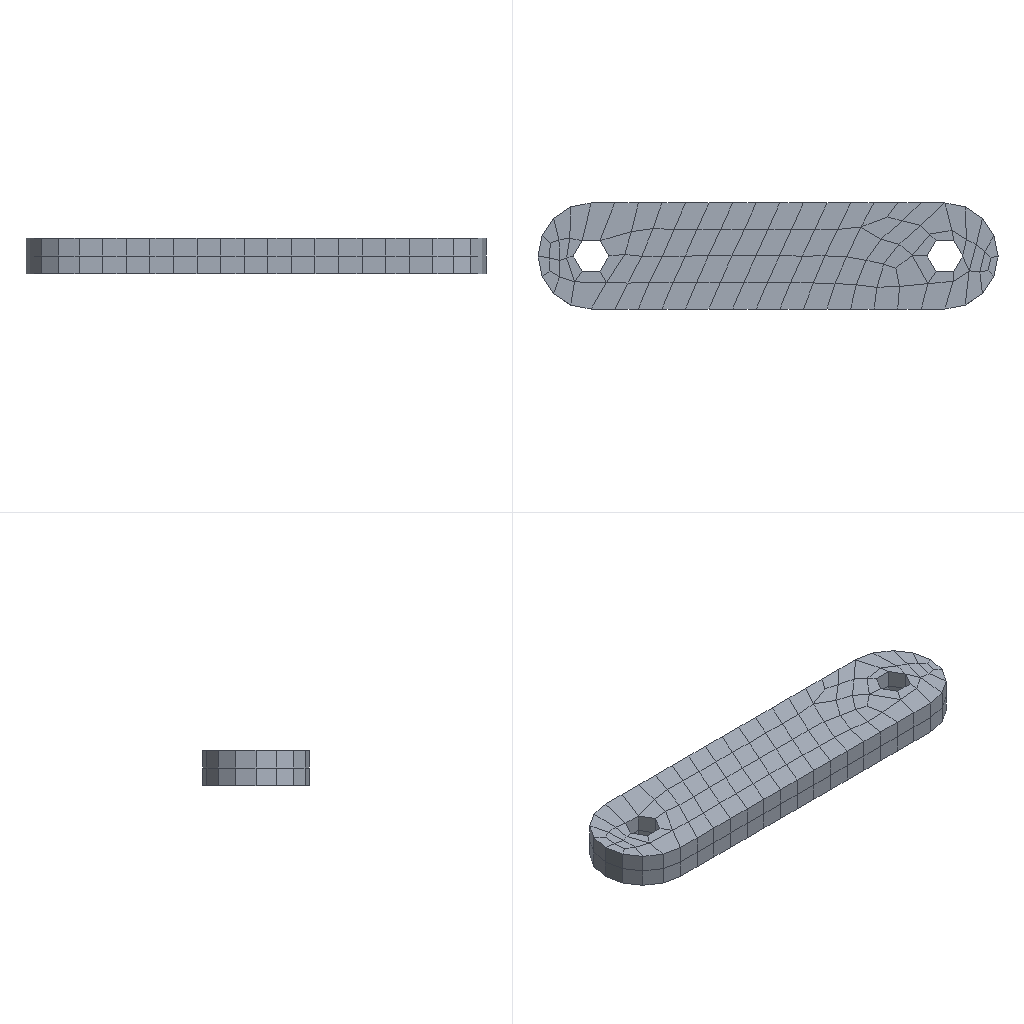Simulation study | ansys workbench
Ansys APDL input file, long lists of numbers shortened:
/batch
/config,noeldb,1     ! force off writing results to database
*get,_wallstrt,active,,time,wall
! ANSYS input file written by Workbench version 2022 R1
! File used for geometry attach: F:\ansys（分析文件汇总)\连杆和曲柄有限元分析\舵机架.STEP
/title,wbnew--____ (B5)
! ****** Begin Custom Load Command Snippet ******
/COM, ACT Extensions:
/COM,     LSDYNA, 2021.1
/COM,
! ****** End   Custom Load Command Snippet ******
*DIM,_wb_ProjectScratch_dir,string,248
_wb_ProjectScratch_dir(1) = 'C:\Users\Administrator\AppData\Local\Temp\WB_Administrator_9524_2\_ProjectScratch\ScrD814\'
*DIM,_wb_SolverFiles_dir,string,248
_wb_SolverFiles_dir(1) = 'C:\Users\Administrator\AppData\Local\Temp\WB_Administrator_9524_2\wbnew_files\dp0\SYS\MECH\'
*DIM,_wb_userfiles_dir,string,248
_wb_userfiles_dir(1) = 'C:\Users\Administrator\AppData\Local\Temp\WB_Administrator_9524_2\wbnew_files\user_files\'
/com,--- Data in consistent NMM units. See Solving Units in the help system for more information.
/units,MPA
/nopr
/wb,file,start              !  signify a WB generated input file
/prep7
! Turn off shape checking because checks already performed inside WB mesher.
! See help system for more information.
SHPP,OFF,,NOWARN
/nolist
etcon,set             ! allow ANSYS to choose best KEYOP's for 180x elements, resets any applicable keyopt to MAPDL defaults
/com,*********** Nodes for the whole assembly ***********
nblock,3,,114635
(1i9,3e20.9e3)
        1     5.800000000E+00     2.000000000E+01    -4.000000000E+00
! (104213 more lines like these left out)
-1
/wb,elem,start            !  set before creation of elements
/com,*********** Elements for Body 1 "___-FreeParts|____-____5" ***********
et,1,187
eblock,19,solid,,30033
(19i9)
        1        1        1        1        0        0        0        0       10        0    29225    57461    59689    58819    57715    94284   102448    94278    94275
! (60065 more lines like these left out)
-1
/com,*********** Elements for Body 2 "___-FreeParts|____-____1" ***********
et,2,187
eblock,19,solid,,29224
(19i9)
        2        2        2        2        0        0        0        0       10        0        1     6994     7254     8134     7776    47665    49608    47675    47673
! (58447 more lines like these left out)
-1
/wb,elem,end               !  done creating elements
/com,*********** Send User Defined Coordinate System(s) ***********
csys,0
toffst,273.15,  ! Temperature offset from absolute zero
/com,*********** Set Reference Temperature ***********
tref,22.
/wb,mat,start              !  starting to send materials
/com,*********** Send Materials ***********
Temperature = 'TEMP' ! Temperature
MP,DENS,1,1.25e-09,	! tonne mm^-3
MP,ALPX,1,1.2e-05,	! C^-1
MP,C,1,434000000,	! mm^2 s^-2 C^-1
MP,KXX,1,60.5,	! tonne mm s^-3 C^-1
MP,RSVX,1,0.00017,	! ohm mm
MP,EX,1,3000,	! tonne s^-2 mm^-1
MP,NUXY,1,0.3,
MP,MURX,1,10000,
Temperature = 'TEMP' ! Temperature
MP,DENS,2,1.25e-09,	! tonne mm^-3
MP,ALPX,2,1.2e-05,	! C^-1
MP,C,2,434000000,	! mm^2 s^-2 C^-1
MP,KXX,2,60.5,	! tonne mm s^-3 C^-1
MP,RSVX,2,0.00017,	! ohm mm
MP,EX,2,3000,	! tonne s^-2 mm^-1
MP,NUXY,2,0.3,
MP,MURX,2,10000,
/wb,mat,end                !  done sending materials
!************************* Model Summary ********************
!___-FreeParts|____-____5,	PLA,	matid,	1
!___-FreeParts|____-____1,	PLA,	matid,	2
!************************* End Model Summary ********************
! get the diagonal of the bounding box. Needed later for other things
*get,_xmin,node,,mnloc,x
*get,_ymin,node,,mnloc,y
*get,_zmin,node,,mnloc,z
*get,_xmax,node,,mxloc,x
*get,_ymax,node,,mxloc,y
*get,_zmax,node,,mxloc,z
_ASMDIAG=(_xmax-_xmin)*(_xmax-_xmin)+(_ymax-_ymin)*(_ymax-_ymin)+(_zmax-_zmin)*(_zmax-_zmin)
_ASMDIAG=SQRT(_ASMDIAG)
/wb,contact,start          !  starting to send contact
/com,*********** Create Contact "接触区域" ***********
/com,            Real Constant Set For Above Contact Is 4 & 3
*set,tid,4
*set,cid,3
r,tid
r,cid
et,tid,170
et,cid,174
eblock,10,,,2211
(15i9)
    83154        4        4        4        0    51462    51466    52017    52017    60587    60624    52017    60589
! (2210 more lines like these left out)
-1
eblock,10,,,2211
(15i9)
    85365        3        3        3        0    51462    51466    52017    52017    60587    60624    52017    60589
! (2210 more lines like these left out)
-1
eblock,10,,,2299
(15i9)
    87576        3        4        3        0     3099     3412     3676     3676    25484    27890     3676    25487
! (2298 more lines like these left out)
-1
eblock,10,,,2299
(15i9)
    89875        4        3        4        0     3099     3412     3676     3676    25484    27890     3676    25487
! (2298 more lines like these left out)
-1
keyo,cid,8,2               ! auto create asymmetric contact (from Program Controlled setting)
keyo,cid,10,0              ! adjust contact stiffness each NR iteration (from Program Controlled setting)
keyo,cid,12,5              ! bonded always
keyo,cid,18,1              ! small sliding turned on by application
keyo,cid,2,0               ! augmented Lagrange (from Program Controlled setting)
keyo,cid,4,0               ! on Gauss point (from Program Controlled setting)
keyo,cid,9,1               ! ignore initial gaps/penetration
keyo,cid,7,0               ! No Prediction
rmod,tid,3,10.      ! FKN
rmod,tid,5,0.       ! ICONT
rmod,tid,6,0.       ! PINB
rmod,tid,10,0.      ! CNOF
rmod,tid,12,0.      ! FKT
rmod,tid,36,29      ! WB DSID
rmod,cid,3,10.      ! FKN
rmod,cid,5,0.       ! ICONT
rmod,cid,6,0.       ! PINB
rmod,cid,10,0.      ! CNOF
rmod,cid,12,0.      ! FKT
rmod,cid,36,29      ! WB DSID
nsel,all
esel,all
/wb,contact,end            !  done creating contacts
/golist
/wb,load,start             !  starting to send loads
/com,*********** Fixed Supports ***********
CMBLOCK,_FIXEDSU,NODE,     5902
(8i10)
       125       126       127       128       129       130       131       132
! (737 more lines like these left out)
cmsel,s,_FIXEDSU
d,all,all
nsel,all
/com,*********** Define Force Using Surface Effect Elements ***********
local,12,0,0.,0.,0.,0.,0.,0.
csys,0
et,5,154
eblock,10,,,1333
(15i9)
    92174        5        5        5       12     5136     5246     5210     5210    36742    37269     5210    36740
! (1332 more lines like these left out)
-1
esel,s,type,,5
keyop,5,2,1                ! Apply load in local coordinate system
keyop,5,7,1                ! Use original area so load is constant in large deformation
esel,all
/com,*********** Define Force Using Surface Effect Elements ***********
local,13,0,0.,0.,0.,0.,0.,0.
csys,0
et,6,154
eblock,10,,,498
(15i9)
    93507        6        6        6       13     4437     4492     4484     4484    32843    33162     4484    32840
! (497 more lines like these left out)
-1
esel,s,type,,6
keyop,6,2,1                ! Apply load in local coordinate system
keyop,6,7,1                ! Use original area so load is constant in large deformation
esel,all
/gst,on,on
fini
*get,_numnode,node,0,count
*get,_numelem,elem,0,count
*get, _MAXELEMNUM, elem, 0, NUM, MAX
*get, _MAXNODENUM, node, 0, NUM, MAX
*get, _MAXELEMTYPE, etyp, 0, NUM, MAX
*get, _MAXREALCONST, real, 0, NUM, MAX
/go
/wb,load,end               !  done creating loads
/com,--- Number of total nodes = %_numnode%
/com,--- Number of contact elements = 10851
/com,--- Number of spring elements = 0
/com,--- Number of bearing elements = 0
/com,--- Number of solid elements = 59257
/com,--- Number of condensed parts = 0
/com,--- Number of total elements = %_numelem%
*get,_wallbsol,active,,time,wall
/com,****************************************************************************
/com,*************************    SOLUTION       ********************************
/com,****************************************************************************
/solu
antype,0                   ! static analysis
_thickRatio=  1     ! Ratio of thick parts in the model
eqsl,pcg,1e-8,,,,,,1
cntr,print,1               ! print out contact info and also make no initial contact an error
dmpoption,emat,no             ! Don't combine emat file for DANSYS
dmpoption,esav,no             ! Don't combine esav file for DANSYS
nldiag,cont,iter           ! print out contact info each equilibrium iteration
rescontrol,,none                 ! Do not keep any restart files
/com,****************************************************
/com,******************* SOLVE FOR LS 1 OF 1 ****************
esel,s,type,,5
nsle
sfe,all,1,pres,1,0.
sfe,all,2,pres,1,-7.89154600444757e-004
sfe,all,3,pres,1,0.
esel,s,type,,6
nsle
sfe,all,1,pres,1,0.
sfe,all,2,pres,1,9.87286615982099e-003
sfe,all,3,pres,1,0.
nsel,all
esel,all
/nopr
/gopr
nsub,1,1,1
time,1.
outres,erase
outres,all,none
outres,nsol,all,
outres,rsol,all
outres,eangl,all
outres,etmp,all
outres,veng,all
outres,strs,all,
outres,epel,all,
outres,eppl,all,
outres,cont,all,
! *********** WB SOLVE COMMAND ***********
! check interactive state
*get,ANSINTER_,active,,int
*if,ANSINTER_,ne,0,then
/eof
*endif
solve
/com *************** Write FE CONNECTORS *********
CEWRITE,file,ce,,INTE
/com,****************************************************
/com,*************** FINISHED SOLVE FOR LS 1 *************
*get,_wallasol,active,,time,wall
/nopr
*get,_numnode,node,0,count
*get,_numelem,elem,0,count
*get, _MAXELEMNUM, elem, 0, NUM, MAX
*get, _MAXNODENUM, node, 0, NUM, MAX,,,INTERNAL
*get, _MAXELEMTYPE, etyp, 0, NUM, MAX
*get, _MAXREALCONST, real, 0, NUM, MAX
/gopr
*get,_PCGITER,active,,solu,cgiter
/post1
xmlo,ENCODING,ISO-8859-1
xmlo,parm
/xml,parm,xml
fini
/gopr
*get,_walldone,active,,time,wall
_preptime=(_wallbsol-_wallstrt)*3600
_solvtime=(_wallasol-_wallbsol)*3600
_posttime=(_walldone-_wallasol)*3600
_totaltim=(_walldone-_wallstrt)*3600
*get,_dlbratio,active,0,solu,dlbr
*get,_combtime,active,0,solu,comb
*get,_ssmode,active,0,solu,ssmm
*get,_ndofs,active,0,solu,ndof
*get,_sol_end_time,active,0,set,time
*if,_sol_end_time,eq,1.,then
/fclean				!clean distributed files
*endif
/com,--- Total number of nodes = %_numnode%
/com,--- Total number of elements = %_numelem%
/com,--- Element load balance ratio = %_dlbratio%
/com,--- Time to combine distributed files = %_combtime%
/com,--- Sparse memory mode = %_ssmode%
/com,--- Number of DOF = %_ndofs%
/wb,file,end               ! done with WB generated input